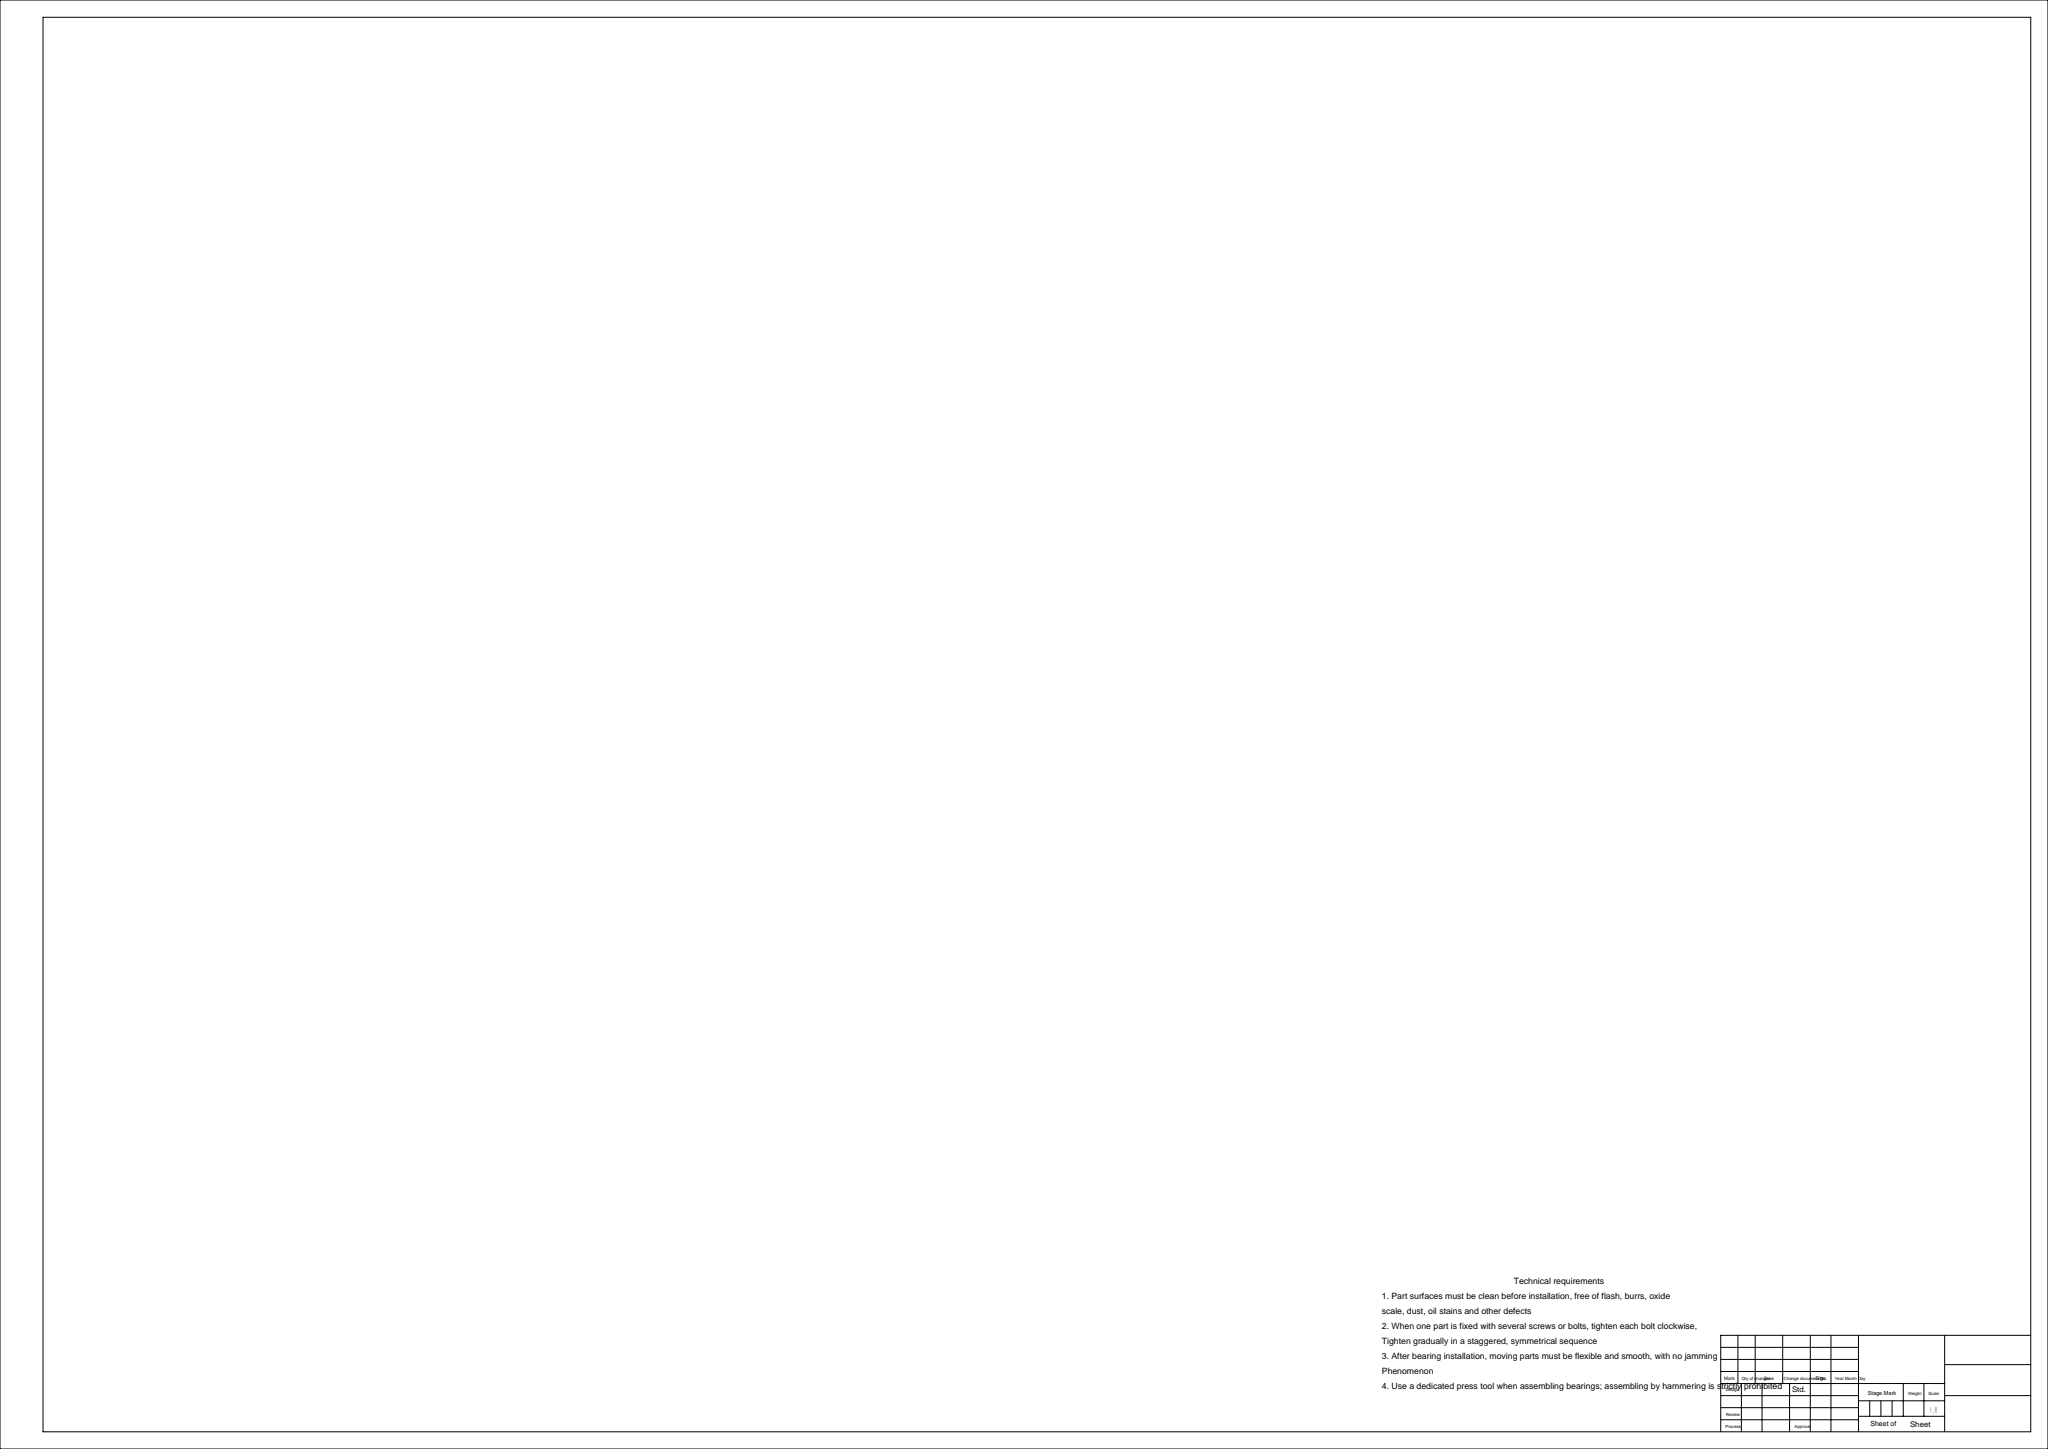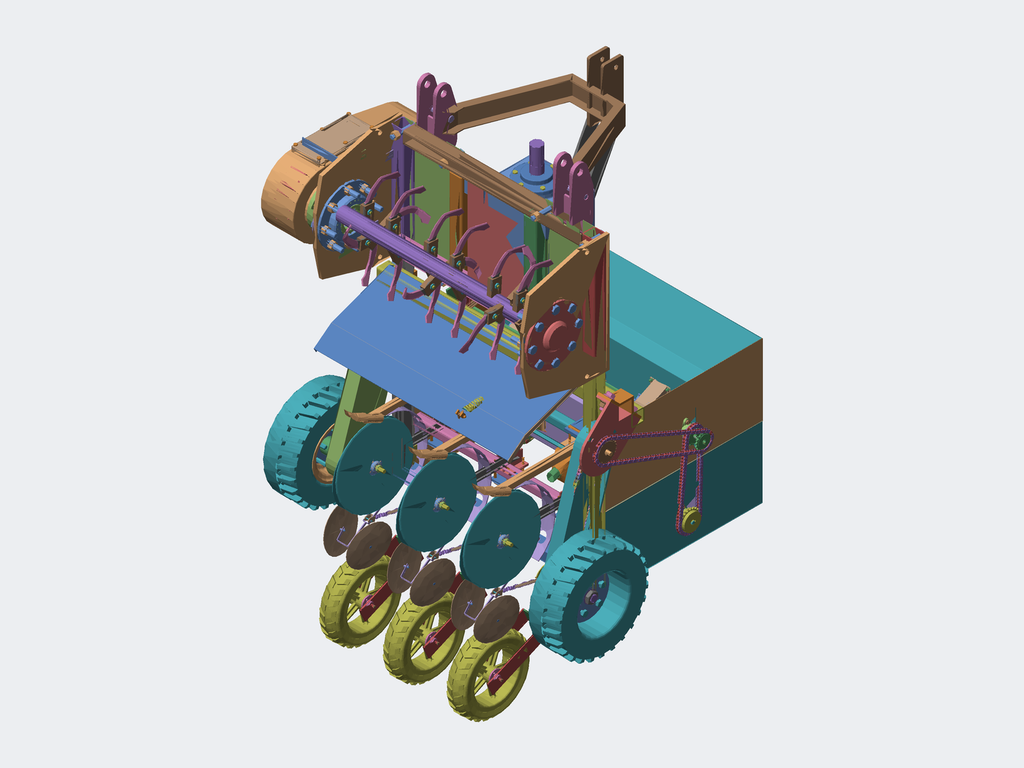Assembly | SolidWorks | 209 different items | 1308 placed
Parts list (item | name | quantity | parent item | size | volume | features):
1 | (subassembly) | x1 | - | - | - | features CompositeCurve 6
2 | (subassembly) | x1 | - | 866 x 574.882 x 353.001 mm | 3236381 mm3 | features ReferencePattern 8, LocalLPattern 1
3 | (subassembly) | x1 | - | 866 x 581.033 x 134.332 mm | 1380836 mm3 | -
4 | (subassembly) | x3 | in 5 | 163 x 229.711 x 140 mm | 1064629 mm3 | features CompositeCurve 9, ReferencePattern 6, LocalCirPattern 2, MirrorCompFeat 1
5 | (subassembly) | x1 | - | - | 6401215 mm3 | features ReferencePattern 29, LocalLPattern 4, CompositeCurve 2, MirrorCompFeat 2, LocalCirPattern 1
6 | (subassembly) | x1 | - | - | - | features CompositeCurve 20
7 | (subassembly) | x3 | in 8 | 130 x 170 x 165 mm | 426747 mm3 | -
8 | (subassembly) | x1 | - | 338 x 752 x 1133 mm | 4481337 mm3 | features ReferencePattern 18, LocalLPattern 3, CompositeCurve 2, LocalCirPattern 1
9 | (subassembly) | x1 | - | - | - | -
10 | (subassembly) | x1 | - | - | - | features ReferencePattern 8, LocalCirPattern 2, CompositeCurve 1
11 | (subassembly) | x1 | - | - | 19308799 mm3 | features ReferencePattern 66, LocalCirPattern 6, LocalLPattern 2, CompositeCurve 1, MirrorCompFeat 1
12 | (subassembly) | x3 | in 18 | 109 x 450 x 60 mm | 238814 mm3 | features CompositeCurve 2, MirrorCompFeat 2, ReferencePattern 2
13 | (subassembly) | x3 | - | 168.807 x 189.61 x 405.761 mm | 223720 mm3 | features CompositeCurve 6, MirrorCompFeat 2, ReferencePattern 2
14 | (subassembly) | x1 | in 5 | 105 x 105 x 103.075 mm | 214366 mm3 | features CompositeCurve 2
15 | (subassembly) | x1 | - | - | 206432 mm3 | features ReferencePattern 96, Belt 1, LocalChainPattern 1
16 | (subassembly) | x1 | - | - | 364523 mm3 | features ReferencePattern 73, Belt 1, LocalChainPattern 1
17 | (subassembly) | x74 | in 16 | 36.351 x 17.823 x 16.175 mm | 2555 mm3 | -
18 | (subassembly) | x3 | - | 130 x 571.206 x 341.736 mm | 2047297 mm3 | features CompositeCurve 1, MirrorCompFeat 1, ReferencePattern 1
19 | (subassembly) | x1 | - | 510.982 x 565.982 x 357 mm | 19755634 mm3 | features ReferencePattern 5, CompositeCurve 3, LocalCirPattern 1
20 | (subassembly) | x35 | in 21 | - | - | -
21 | (subassembly) | x1 | - | 975 x 434.394 x 418.8 mm | 2976475 mm3 | features ReferencePattern 52, CompositeCurve 10, LocalLPattern 4, LocalCirPattern 2, AEMSimFeature 1
22 | (subassembly) | x3 | in 2 | 353.001 x 130.927 x 574.882 mm | 819203 mm3 | features ReferencePattern 7, CompositeCurve 3, MirrorCompFeat 2
23 | (subassembly) | x1 | in 10 | - | - | features CompositeCurve 47, AEMSimFeature 1
24 | (subassembly) | x49 | in 15 | 25.03 x 12.33 x 14.51 mm | 799.359 mm3 | -
25 | (subassembly) | x1 | in 10 | - | - | features CompositeCurve 84, AEMSimFeature 1, Belt 1
26 | - | x2 | in 19 | 95.5 x 93.873 x 2.5 mm | 3834 mm3 | features Extrusion 1
27 | - | x2 | in 23, 25 | - | - | features ICE 2, Extrusion 1, SweepThread 1
28 | - | x1 | in 25 | 660 x 205 x 60 mm | 1732722 mm3 | features ICE 2, Extrusion 1
29 | - | x2 | in 23, 25 | 250 x 200 x 60 mm | 547961 mm3 | features ICE 3, Cut 1, Extrusion 1
30 | - | x1 | in 23 | - | 127327 mm3 | features Boss 3, CurvePattern 2, Chamfer 1, CompositeCurve 1, Extrusion 1, MirrorPattern 1, MirrorSolid 1
31 | - | x2 | in 23, 25 | 32 x 32 x 76 mm | 32270 mm3 | features Helix 1, Sweep 1
32 | - | x3 | in 4 | 115 x 115 x 40 mm | 37157 mm3 | features ICE 5, Extrusion 1, RefAxis 1, RefPoint 1
33 | - | x3 | in 4 | 120 x 120 x 7.5 mm | 38485 mm3 | features RefAxis 4, ICE 2, Extrusion 1
34 | - | x3 | in 4 | 98.826 x 98.952 x 30 mm | 216398 mm3 | features Extrusion 1, ICE 1
35 | - | x3 | in 4 | 100 x 100 x 65 mm | 446877 mm3 | features ICE 2, CirPattern 1, Extrusion 1
36 | - | x2 | - | 260 x 260 x 30 mm | 552397 mm3 | features ICE 2, Chamfer 1, Extrusion 1
37 | - | x2 | in 19 | 49 x 53.209 x 1.5 mm | 876.142 mm3 | features Extrusion 1
38 | - | x1 | - | 260 x 260 x 10 mm | 427257 mm3 | features Extrusion 1, ICE 1
39 | - | x246 | in 17, 24 | 25.03 x 12.33 x 1.665 mm | 399.679 mm3 | features Cut 1, Extrusion 1
40 | - | x1 | in 10 | 26 x 26 x 10 mm | 3542 mm3 | features Extrusion 1
41 | - | x1 | in 21 | 975 x 80 x 80 mm | 1427415 mm3 | features Chamfer 3, ICE 3, Extrusion 1, Fillet 1
42 | - | x11 | in 21 | 167.64 x 57.038 x 10 mm | 39018 mm3 | features Blend 1, Extrusion 1
43 | - | x18 | in 21 | 186.248 x 81.99 x 35.546 mm | 40697 mm3 | features ICE 2, Chamfer 1, CombineBodies 1, Deform 1, DeleteBody 1, Extrusion 1, FillRefSurface 1, MirrorPattern 1, RefCurve 1, Split 1, SurfCut 1, SweepCut 1
44 | - | x1 | in 25 | 64 x 64 x 195 mm | 414709 mm3 | features ICE 5, SweepThread 2, Chamfer 1, Extrusion 1
45 | - | x3 | in 3 | 134.332 x 42 x 580 mm | 122750 mm3 | features ICE 5, Blend 1, Extrusion 1
46 | - | x12 | in 2, 3 | 100 x 70 x 10 mm | 18547 mm3 | features Helix 2, SweepCut 2, Fillet 1, Sweep 1
47 | - | x9 | in 2, 3 | 100 x 80 x 10 mm | 76199 mm3 | features Extrusion 1
48 | - | x2 | in 19 | 34 x 14 x 9 mm | 3893 mm3 | features Extrusion 1, Fillet 1
49 | - | x1 | in 2 | 866 x 40 x 40 mm | 463134 mm3 | features WeldMemberFeat 1, WeldmentFeature 1
50 | - | x1 | in 3 | 866 x 40 x 40 mm | 463134 mm3 | features WeldMemberFeat 1, WeldmentFeature 1
51 | - | x3 | - | 12 x 280 x 12 mm | 31370 mm3 | features Extrusion 1, ICE 1, MirrorPattern 1
52 | - | x1 | - | 52.165 x 415.629 x 914 mm | 1472368 mm3 | features FlatPattern 2, SMBaseFlange 2, SheetMetal 2, ICE 1, MirrorSolid 1
53 | - | x5 | - | 130 x 60 x 57 mm | 96959 mm3 | features Cut 1, Extrusion 1, Fillet 1, ICE 1, LPattern 1
54 | - | x2 | - | 20 x 20 x 20 mm | 2749 mm3 | features Extrusion 1
55 | - | x4 | - | 16 x 26 x 5 mm | 1550 mm3 | features Extrusion 1
56 | - | x2 | - | 32 x 32 x 306 mm | 76200 mm3 | features Helix 1, RefAxis 1, Sweep 1
57 | - | x3 | in 22 | 328.42 x 176 x 80 mm | 44356 mm3 | features ICE 4, ExtruRefSurface 1, Thicken 1
58 | - | x1 | in 14 | 105 x 105 x 30 mm | 95976 mm3 | features ICE 2, Extrusion 1
59 | - | x1 | - | 10 x 5 x 5 mm | 221.448 mm3 | features Extrusion 1, Fillet 1
60 | - | x3 | in 7 | 22 x 22 x 165 mm | 19772 mm3 | features Extrusion 1, ICE 1
61 | - | x3 | in 7 | 68 x 68 x 120 mm | 167321 mm3 | features ICE 2, Extrusion 1
62 | - | x3 | in 7 | 130 x 170 x 96 mm | 239654 mm3 | features ICE 8, Blend 1, Extrusion 1, Shell 1
63 | - | x1 | in 8 | 15 x 15 x 1130 mm | 199245 mm3 | features ICE 3, Extrusion 1
64 | - | x3 | in 4 | 163 x 141.711 x 140 mm | 274719 mm3 | features ICE 8, Fillet 6, Extrusion 1, Shell 1
65 | - | x1 | in 5 | 45 x 45 x 15 mm | 8861 mm3 | features ICE 2, Extrusion 1
66 | - | x1 | in 14 | 48 x 48 x 7 mm | 4020 mm3 | features Extrusion 1, ICE 1
67 | - | x1 | in 14 | 55 x 55 x 10 mm | 12395 mm3 | features Extrusion 1
68 | - | x1 | in 14 | 75 x 75 x 103 mm | 101976 mm3 | features ICE 4, Extrusion 1, Shell 1
69 | - | x1 | in 5 | 15 x 15 x 1090 mm | 192288 mm3 | features ICE 2, Extrusion 1, Fillet 1
70 | - | x2 | in 5, 8 | 14 x 5 x 5 mm | 320.899 mm3 | features Extrusion 1, Fillet 1
71 | - | x1 | in 8 | 105 x 105 x 30 mm | 95568 mm3 | features ICE 2, Extrusion 1
72 | - | x1 | in 8 | 48 x 48 x 7 mm | 4020 mm3 | features Extrusion 1, ICE 1
73 | - | x1 | in 8 | 55 x 55 x 10 mm | 12395 mm3 | features Extrusion 1
74 | - | x1 | in 8 | 75 x 75 x 103 mm | 101976 mm3 | features ICE 4, Extrusion 1, Shell 1
75 | - | x2 | - | 580 x 21 x 21 mm | 191345 mm3 | features ICE 4, Revolution 1
76 | - | x3 | in 22 | 100 x 60 x 80 mm | 110678 mm3 | features ICE 3, Extrusion 1, MirrorPattern 1
77 | - | x3 | in 4 | 42.184 x 46.319 x 39 mm | 4653 mm3 | features Extrusion 1, ICE 1, Shell 1, Sweep 1
78 | - | x2 | - | 260 x 260 x 41 mm | 859714 mm3 | features ICE 3, Chamfer 2, CirPattern 1, Extrusion 1, Fillet 1
79 | - | x1 | - | 960 x 60 x 1436 mm | 5295924 mm3 | features ICE 2, MirrorPattern 2, LPattern 1, WeldMemberFeat 1, WeldmentFeature 1
80 | - | x6 | in 12 | 5 x 300 x 60 mm | 89607 mm3 | features Extrusion 1, ICE 1
81 | - | x2 | in 11 | 16 x 80 x 80 mm | 32317 mm3 | features Revolution 6, CirPattern 2, RevCut 2, MirrorPattern 1
82 | - | x3 | in 12 | 99 x 5 x 60 mm | 29700 mm3 | features Extrusion 1
83 | - | x6 | in 12 | 2 x 150 x 50 mm | 14950 mm3 | features ICE 3, Extrusion 1
84 | - | x12 | in 5 | 50 x 9.031 x 30 mm | 3952 mm3 | features ICE 2, Extrusion 1
85 | - | x3 | in 4 | 80 x 45 x 5 mm | 16384 mm3 | features ICE 3, Extrusion 1, LPattern 1
86 | - | x2 | - | 80 x 40 x 40 mm | 37542 mm3 | features Extrusion 1, ICE 1, MirrorSolid 1
87 | - | x3 | - | 34 x 10 x 14 mm | 1005 mm3 | features Extrusion 1, ICE 1, MirrorSolid 1
88 | - | x2 | - | 530 x 2 x 280 mm | 290567 mm3 | features ICE 2, Extrusion 1
89 | - | x1 | - | 415.5 x 2 x 290 mm | 240990 mm3 | features Extrusion 1
90 | - | x1 | in 5 | 337 x 313.5 x 920 mm | 1609120 mm3 | features MirrorPattern 2, FlatPattern 1, ICE 1, SMBaseFlange 1, SheetMetal 1
91 | - | x1 | in 5 | 32 x 752 x 333 mm | 518361 mm3 | features FlatPattern 1, ICE 1, SMBaseFlange 1, SheetMetal 1
92 | - | x1 | in 10 | 5 x 24 x 24 mm | 880.809 mm3 | features Revolution 5, CirPattern 2, RevCut 2
93 | - | x1 | in 5 | 32 x 752 x 333 mm | 518481 mm3 | features ICE 2, FlatPattern 1, SMBaseFlange 1, SheetMetal 1
94 | - | x3 | in 22 | 35 x 12 x 415 mm | 167863 mm3 | features Extrusion 1, ICE 1
95 | - | x1 | - | 40 x 10 x 69.01 mm | 22746 mm3 | features Extrusion 1
96 | - | x1 | - | 40 x 10 x 66.57 mm | 21770 mm3 | features Extrusion 1
97 | - | x1 | in 8 | 32 x 752 x 337 mm | 524643 mm3 | features FlatPattern 1, ICE 1, SMBaseFlange 1, SheetMetal 1
98 | - | x1 | in 8 | 32 x 752 x 337 mm | 524731 mm3 | features ICE 2, FlatPattern 1, SMBaseFlange 1, SheetMetal 1
99 | - | x1 | - | 60 x 60 x 200 mm | 299813 mm3 | features ICE 2, Extrusion 1
100 | - | x1 | in 8 | 337 x 313.5 x 920 mm | 1639360 mm3 | features MirrorPattern 2, FlatPattern 1, ICE 1, SMBaseFlange 1, SheetMetal 1
101 | - | x3 | - | 16 x 16 x 176 mm | 26240 mm3 | features Helix 1, RefAxis 1, Sweep 1
102 | - | x3 | - | 20 x 232 x 20 mm | 18563 mm3 | features ICE 5, Extrusion 1
103 | - | x6 | in 18 | 9 x 30 x 30 mm | 4054 mm3 | features Revolution 5, CirPattern 2, RevCut 2
104 | - | x3 | in 13 | 138.916 x 10 x 352 mm | 16665 mm3 | features ICE 6, Extrusion 1, MirrorPattern 1
105 | - | x6 | in 13 | 189.61 x 7.325 x 189.61 mm | 102683 mm3 | features Fillet 1, ICE 1, Revolution 1
106 | - | x3 | in 18 | 87.248 x 341.454 x 341.945 mm | 1756971 mm3 | features CirPattern 5, ICE 5, Fillet 3, Chamfer 2, Revolution 2
107 | - | x6 | in 18 | 60 x 60 x 18.5 mm | 16720 mm3 | features ICE 2, Extrusion 1
108 | - | x2 | in 23, 25 | 240 x 240 x 140 mm | 3010326 mm3 | features ICE 4, Extrusion 1, Fillet 1, MirrorPattern 1
109 | - | x2 | in 23, 25 | 440 x 440 x 140 mm | 12462431 mm3 | features BlendCut 2, CirPattern 2, Extrusion 1, Fillet 1
110 | - | x1 | in 23 | 48 x 48 x 10 mm | 5529 mm3 | features Extrusion 1
111 | - | x1 | in 25 | 48 x 48 x 10 mm | 5529 mm3 | features Extrusion 1
112 | - | x3 | in 18 | 10 x 10 x 130 mm | 9964 mm3 | features Extrusion 1, ICE 1
113 | - | x2 | - | 300 x 98 x 92 mm | 689780 mm3 | features ICE 2, Extrusion 1, Fillet 1, LPattern 1
114 | - | x4 | in 19 | 20 x 90 x 90 mm | 55631 mm3 | features Revolution 6, CirPattern 2, RevCut 2, MirrorPattern 1
115 | - | x1 | - | 550 x 539.301 x 285 mm | 1145728 mm3 | features ICE 3, MirrorSolid 3, ExtruRefSurface 1, Thicken 1
116 | - | x2 | - | 341.614 x 178.454 x 10 mm | 201659 mm3 | features Extrusion 1
117 | - | x3 | - | 30 x 95 x 165 mm | 47978 mm3 | features ICE 1, WeldMemberFeat 1, WeldmentFeature 1
118 | - | x7 | - | 53.74 x 83.25 x 20 mm | 11198 mm3 | features ICE 2, Extrusion 1
119 | - | x3 | - | 17 x 17 x 154 mm | 7958 mm3 | features Helix 1, RefAxis 1, Sweep 1
120 | - | x2 | in 11 | 20 x 90 x 90 mm | 55631 mm3 | features Revolution 6, CirPattern 2, RevCut 2, MirrorPattern 1
121 | - | x3 | - | 4 x 4 x 50 mm | 613.938 mm3 | features Chamfer 1, Cut 1, Extrusion 1
122 | - | x1 | in 11 | 21 x 100 x 100 mm | 73176 mm3 | features Revolution 6, CirPattern 2, RevCut 2, MirrorPattern 1
123 | - | x3 | in 11 | 25 x 100 x 100 mm | 96597 mm3 | features Revolution 6, CirPattern 2, RevCut 2, MirrorPattern 1
124 | - | x1 | in 5 | 13.2 x 35 x 35 mm | 6194 mm3 | features Revolution 4, CirPattern 1
125 | - | x2 | - | 26 x 140 x 140 mm | 191182 mm3 | features Revolution 3, CirPattern 1
126 | - | x6 | in 22 | 22 x 40 x 40 mm | 10628 mm3 | features Revolution 3, RevCut 2, CirPattern 1
127 | - | x1 | in 10 | 26.17 x 22.664 x 15.9 mm | 3864 mm3 | features Cut 2, Chamfer 1, Extrusion 1
128 | - | x26 | - | 32.95 x 28.536 x 19 mm | 7406 mm3 | features Cut 2, Chamfer 1, Extrusion 1
129 | - | x4 | in 19 | 36.4 x 18.475 x 16 mm | 3739 mm3 | features RevCut 4, Chamfer 1, Extrusion 1, Fillet 1, LPattern 1, Revolution 1
130 | - | x14 | in 19 | 41.4 x 18.475 x 16 mm | 4131 mm3 | features RevCut 4, Chamfer 1, Extrusion 1, Fillet 1, LPattern 1, Revolution 1
131 | - | x31 | in 11 | 37.5 x 20.785 x 18 mm | 5444 mm3 | features RevCut 4, Chamfer 1, Extrusion 1, Fillet 1, LPattern 1, Revolution 1
132 | - | x2 | - | 34.5 x 14 x 14 mm | 2728 mm3 | features Chamfer 1, Cut 1, Fillet 1, Revolution 1
133 | - | x40 | in 5, 8 | 25.3 x 15.011 x 13 mm | 1760 mm3 | features RevCut 4, Chamfer 1, Extrusion 1, Fillet 1, LPattern 1, Revolution 1
134 | - | x6 | in 11 | 35.3 x 15.011 x 13 mm | 2262 mm3 | features RevCut 4, Chamfer 1, Extrusion 1, Fillet 1, LPattern 1, Revolution 1
135 | - | x10 | in 10 | 75 x 27.713 x 24 mm | 17949 mm3 | features RevCut 4, Chamfer 1, Extrusion 1, Fillet 1, LPattern 1, Revolution 1
136 | - | x24 | - | 102.5 x 34.641 x 30 mm | 37820 mm3 | features RevCut 4, Chamfer 1, Extrusion 1, Fillet 1, LPattern 1, Revolution 1
137 | - | x18 | in 21 | 37.5 x 20.785 x 18 mm | 5444 mm3 | features RevCut 4, Chamfer 1, Extrusion 1, Fillet 1, LPattern 1, Revolution 1
138 | - | x18 | in 21 | 17.386 x 20.03 x 10.8 mm | 1566 mm3 | features Cut 2, Chamfer 1, Extrusion 1
139 | - | x12 | in 5 | 12.482 x 14.38 x 4 mm | 327.094 mm3 | features Cut 2, Chamfer 1, Extrusion 1
140 | - | x6 | in 22 | 23.219 x 26.75 x 8 mm | 2049 mm3 | features Cut 2, Chamfer 1, Extrusion 1
141 | - | x4 | in 5, 8 | 26 x 16 x 16 mm | 2579 mm3 | features Cut 1, LPattern 1, RevCut 1, Revolution 1
142 | - | x8 | in 5, 8 | 23.9 x 10 x 10 mm | 819.417 mm3 | features Cut 1, LPattern 1, RevCut 1, Revolution 1
143 | - | x2 | - | 124 x 28 x 28 mm | 46998 mm3 | features Chamfer 1, Cut 1, Fillet 1, Revolution 1
144 | - | x24 | in 4 | 16 x 15.8 x 15.673 mm | 989.006 mm3 | features Chamfer 1, Cut 1, LPattern 1, RevCut 1, Revolution 1
145 | - | x2 | in 5, 8 | 99 x 61 x 32.9 mm | 62248 mm3 | features Revolution 5, Boss 2, RevCut 2, CirPattern 1, Cut 1, Extrusion 1
146 | - | x6 | in 4 | 30.97 x 16 x 16 mm | 2140 mm3 | features BlendCut 1, LPattern 1, MirrorPattern 1, RevCut 1, Revolution 1
147 | - | x31 | in 11 | 18.367 x 18.334 x 3.1 mm | 444.091 mm3 | features Extrusion 1
148 | - | x6 | in 11 | 12.277 x 12.254 x 2.1 mm | 135.755 mm3 | features Extrusion 1
149 | - | x24 | in 22 | 14.968 x 7.7 x 7.7 mm | 225.537 mm3 | features Cut 1, Fillet 1, Revolution 1
150 | - | x1 | in 11 | 11 x 18 x 12.702 mm | 898.381 mm3 | features Boss 1, Revolution 1
151 | - | x1 | in 11 | 688 x 310 x 170 mm | 8954968 mm3 | features 3DProfileFeature 6, HoleWzd 6, ICE 6, CirPattern 4, Fillet 3, MirrorPattern 3, Cut 1, Extrusion 1
152 | - | x1 | in 11 | 134.581 x 133.659 x 70 mm | 542357 mm3 | features ICE 2, CirPattern 1, Extrusion 1, RefAxis 1
153 | - | x1 | in 11 | 260.857 x 260.456 x 75 mm | 1917959 mm3 | features ICE 6, Chamfer 5, CirPattern 2, MirrorPattern 2, Extrusion 1, RefAxis 1, RevCut 1
154 | - | x2 | - | 99 x 28 x 28 mm | 37494 mm3 | features Chamfer 1, Cut 1, Fillet 1, Revolution 1
155 | - | x1 | in 11 | 268.959 x 268.959 x 75 mm | 2318333 mm3 | features Chamfer 5, ICE 5, CirPattern 2, Extrusion 1, MirrorPattern 1, RefAxis 1, RevCut 1
156 | - | x1 | in 11 | 62 x 62 x 310 mm | 627287 mm3 | features ICE 4, Chamfer 2, CirPattern 1, Extrusion 1, SweepCut 1
157 | - | x1 | in 11 | 50 x 50 x 160 mm | 295367 mm3 | features ICE 2, Chamfer 1, Extrusion 1
158 | - | x1 | in 11 | 68 x 68 x 312.5 mm | 737851 mm3 | features ICE 4, Chamfer 1, CirPattern 1, Extrusion 1, SweepCut 1
159 | - | x1 | in 11 | 23 x 170 x 170 mm | 323268 mm3 | features Chamfer 1, CirPattern 1, ICE 1, Revolution 1
160 | - | x1 | in 11 | 23 x 190 x 190 mm | 393528 mm3 | features Chamfer 1, CirPattern 1, ICE 1, Revolution 1
161 | - | x1 | in 11 | 40 x 170 x 170 mm | 559070 mm3 | features CirPattern 3, ICE 3, 3DProfileFeature 1, HoleWzd 1, Revolution 1
162 | - | x3 | in 11 | 18 x 170 x 170 mm | 307921 mm3 | features Chamfer 1, CirPattern 1, ICE 1, Revolution 1
163 | - | x2 | in 11 | 63 x 63 x 20 mm | 22197 mm3 | features Chamfer 1, Extrusion 1
164 | - | x2 | in 11 | 63 x 63 x 23.5 mm | 27024 mm3 | features Chamfer 1, Extrusion 1
165 | - | x6 | - | 17.5 x 6 x 6 mm | 227.981 mm3 | features Chamfer 1, Cut 1, Fillet 1, Revolution 1
166 | - | x1 | in 11 | 39 x 190 x 190 mm | 716899 mm3 | features CirPattern 3, ICE 3, 3DProfileFeature 1, HoleWzd 1, Revolution 1
167 | - | x2 | in 11 | 70 x 70 x 17.5 mm | 39425 mm3 | features Chamfer 1, Extrusion 1
168 | - | x1 | in 11 | 270 x 130 x 13 mm | 385260 mm3 | features Extrusion 1, Fillet 1, ICE 1
169 | - | x1 | in 19 | 380 x 380 x 282 mm | 14746846 mm3 | features ICE 13, 3DProfileFeature 3, HoleWzd 3, Fillet 2, Extrusion 1
170 | - | x1 | in 19 | 180 x 180 x 85 mm | 1041607 mm3 | features ICE 4, Fillet 2, 3DProfileFeature 1, CirPattern 1, Extrusion 1, HoleWzd 1
171 | - | x1 | in 19 | 155.563 x 155.563 x 25 mm | 236034 mm3 | features ICE 2, Extrusion 1, Fillet 1
172 | - | x1 | in 19 | 260 x 260 x 75 mm | 829791 mm3 | features ICE 2, Extrusion 1, Fillet 1
173 | - | x1 | in 19 | 329.5 x 60 x 60 mm | 697643 mm3 | features ICE 3, Chamfer 2, Revolution 1
174 | - | x1 | in 19 | 274.5 x 60 x 60 mm | 542135 mm3 | features ICE 3, Chamfer 2, Revolution 1
175 | - | x2 | in 19 | 45.295 x 166.152 x 166.786 mm | 471542 mm3 | features BlendCut 1, CirPattern 1, ICE 1, RefAxis 1, Revolution 1
176 | - | x6 | - | 31.5 x 6 x 6 mm | 403.91 mm3 | features Chamfer 1, Cut 1, Fillet 1, Revolution 1
177 | - | x1 | in 19 | 180 x 180 x 35 mm | 406222 mm3 | features ICE 2, Extrusion 1, Fillet 1
178 | - | x1 | in 25 | 12 x 12 x 19.5 mm | 659.077 mm3 | features Chamfer 2, Cut 2, Boss 1, Extrusion 1, Fillet 1, LPattern 1, RevCut 1
179 | - | x4 | in 23, 25 | 57.7 x 43 x 43 mm | 28324 mm3 | features Fillet 2, RevCut 2, Boss 1, Chamfer 1, Extrusion 1, LPattern 1, Revolution 1
180 | - | x2 | in 23 | 53.116 x 46 x 15 mm | 17946 mm3 | features RevCut 2, Chamfer 1, Extrusion 1, LPattern 1
181 | - | x2 | in 25 | 53.116 x 46 x 15 mm | 18987 mm3 | features RevCut 2, Chamfer 1, Extrusion 1, LPattern 1
182 | - | x1 | in 23 | 26.58 x 18.163 x 15.73 mm | 2955 mm3 | features RevCut 3, Boss 1, Chamfer 1, Extrusion 1, Fillet 1, LPattern 1
183 | - | x4 | in 23, 25 | 42.8 x 42.8 x 20 mm | 13089 mm3 | features RevCut 3, Extrusion 1, Fillet 1, LPattern 1, Revolution 1
184 | - | x3 | in 4 | 121.759 x 70.429 x 82 mm | 20309 mm3 | features MirrorPattern 8, ICE 6, Blend 1, Fillet 1, RefAxis 1, Shell 1
185 | - | x2 | in 23 | 28 x 28 x 10 mm | 3016 mm3 | features Extrusion 1
186 | - | x2 | in 25 | 28 x 28 x 10 mm | 3016 mm3 | features Extrusion 1
187 | - | x6 | in 13 | 28 x 10 x 10 mm | 844.638 mm3 | features Chamfer 1, Cut 1, Fillet 1, Revolution 1
188 | - | x1 | - | 9.37 x 98.633 x 98.858 mm | 54827 mm3 | features Chamfer 3, Cut 2, Revolution 2, CirPattern 1
189 | - | x1 | in 15 | 9.37 x 98.633 x 98.858 mm | 53510 mm3 | features Chamfer 3, Cut 2, Revolution 2, CirPattern 1
190 | - | x2 | in 15, 16 | 9.37 x 73.539 x 73.841 mm | 27730 mm3 | features Chamfer 3, Cut 2, Revolution 2, CirPattern 1
191 | - | x2 | - | 555.5 x 409.096 x 15 mm | 2756721 mm3 | features ICE 5, Chamfer 1, CirPattern 1, Extrusion 1, MirrorPattern 1
192 | - | x123 | in 15, 17 | 24.77 x 12.07 x 16.175 mm | 1756 mm3 | features Boss 2, Chamfer 1, Extrusion 1, MirrorPattern 1
193 | - | x18 | in 21 | 70.526 x 45 x 21 mm | 38872 mm3 | features ICE 3, Extrusion 1
194 | - | x17 | in 21 | 167.64 x 57.038 x 10 mm | 39018 mm3 | features MirrorStock 1
195 | - | x1 | in 23 | 64 x 64 x 195 mm | 414708 mm3 | features ICE 5, SweepThread 2, Chamfer 1, Extrusion 1
196 | - | x2 | - | 200 x 100 x 30 mm | 64241 mm3 | features WeldMemberFeat 1, WeldmentFeature 1
197 | - | x3 | - | 100 x 100 x 30 mm | 41483 mm3 | features WeldMemberFeat 1, WeldmentFeature 1
198 | - | x4 | in 11 | 85.5 x 83.408 x 2.5 mm | 3180 mm3 | features Extrusion 1
199 | - | x2 | - | 30 x 2 x 30 mm | 720.996 mm3 | features Extrusion 1
200 | - | x6 | in 22 | 350 x 350 x 2.3 mm | 217251 mm3 | features ICE 3, Extrusion 1, Sweep 1
201 | - | x3 | in 22 | 130.429 x 28.183 x 19 mm | 26177 mm3 | features ICE 2, Sweep 1
202 | - | x6 | in 22 | 62 x 14 x 62 mm | 4234 mm3 | features ICE 2, Revolution 1
203 | - | x1 | in 10 | 20 x 20 x 120 mm | 27495 mm3 | features ICE 5, Extrusion 1
204 | - | x3 | in 16, 23, 25 | 30 x 98.633 x 98.858 mm | 147727 mm3 | features ICE 2, CirPattern 1, Cut 1, RefAxis 1, Revolution 1
205 | - | x2 | in 23, 25 | 30 x 98.633 x 98.858 mm | 118578 mm3 | features ICE 2, CirPattern 1, Cut 1, RefAxis 1, Revolution 1
206 | - | x1 | in 23 | 660 x 205 x 50 mm | 1585598 mm3 | features ICE 2, Extrusion 1
207 | - | x2 | in 23, 25 | 148.492 x 148.492 x 60 mm | 135835 mm3 | features Cut 1, Extrusion 1, ICE 1
208 | - | x2 | in 23, 25 | 200 x 200 x 20 mm | 321867 mm3 | features Extrusion 1, ICE 1
209 | - | x1 | in 10 | 1200 x 60 x 60 mm | 1025756 mm3 | features WeldMemberFeat 1, WeldmentFeature 1
Mates (type | each side: item.copy, entity, surface, feature), first 427 of 1009 lines:
In the top assembly
Coincident | 79.1 plane | assembly plane | 2 times
Coincident | assembly axis | assembly axis | 15 times
Coincident | assembly face | assembly face | 9 times
Coincident | 79.1 face plane Gb/6728-1986方形空心型钢 060 X 60 X 4(1) | 91.1 face plane Base-Flange 1 | 3 times
Coincident | 79.1 face plane Gb/6728-1986方形空心型钢 060 X 60 X 4(1) | 49.1 face plane Gb/6728-1986方形空心型钢 040 X 40 X 4(1)
Coincident | 79.1 edge | 91.1 edge
Tangent | assembly face | assembly face
Coincident | assembly plane | assembly plane | 3 times
Coincident | 79.1 face plane Gb/6728-1986方形空心型钢 060 X 60 X 4(1) | assembly face | 7 times
Coincident | assembly axis | 199.1 axis
Coincident | assembly face | 199.1 face plane Boss-Extrude 1
Coincident | assembly plane | 79.1 plane
Coincident | 2.1 plane | assembly plane
Coincident | 79.1 face plane Gb/6728-1986方形空心型钢 060 X 60 X 4(1) | 50.1 face plane Gb/6728-1986方形空心型钢 040 X 40 X 4(1)
Coincident | 3.1 plane | assembly plane
Coincident | 79.1 plane | 19.1 plane
Coincident | 79.1 face plane Gb/6728-1986方形空心型钢 060 X 60 X 4(1) | 169.1 face plane Boss-Extrude 1
Coincident | 19.1 plane | assembly plane | 2 times
Coincident | 79.1 edge | 19.1 plane
Coincident | 173.1 axis | 99.1 axis
Coincident | 173.1 edge | 99.1 edge
Coincident | 173.1 face plane Revolve 1 | 99.1 face plane Cut-Extrude 1
Coincident | 99.1 axis | 156.1 axis
Coincident | 99.1 face plane Cut-Extrude 2 | 156.1 face plane Boss-Extrude 4
Coincident | 158.1 axis | 41.1 axis
Coincident | 158.1 face plane Boss-Extrude 3 | 41.1 face plane Boss-Extrude 1
Coincident | 41.1 axis | 191.1 axis
Coincident | 79.1 face plane Gb/6728-1986方形空心型钢 060 X 60 X 4(1) | 191.1 edge
Parallel | assembly plane | 191.1 plane
Coincident | 158.1 axis | 78.1 axis
Coincident | 125.1 axis | 158.1 axis
Coincident | 78.1 face plane Boss-Extrude 1 | 125.1 face plane Base-Revolve
Coincident | 125.2 axis | 36.1 axis
Coincident | 191.1 axis | 36.1 axis
Coincident | 78.2 axis | 36.1 axis
Coincident | 191.1 face plane Boss-Extrude 1 | 36.1 face plane Boss-Extrude 1
Coincident | 158.1 axis | 38.1 axis
Coincident | 78.1 axis | 38.1 axis
Coincident | 19.1 plane | 11.1 plane
Coincident | 191.2 axis | 191.1 axis | 2 times
Coincident | 79.1 face plane Gb/6728-1986方形空心型钢 060 X 60 X 4(1) | 191.2 face plane Boss-Extrude 1
Coincident | 52.1 face plane Mirror 3 | 55.1 face plane Boss-Extrude 1
Parallel | 52.1 edge | 55.1 edge
Coincident | 52.1 face plane Mirror 3 | assembly face
Coincident | 52.1 face plane Mirror 3 | 55.2 face plane Boss-Extrude 1
Parallel | 52.1 edge | 55.2 edge
DistanceDim | 55.1 face plane Boss-Extrude 1 | 55.2 face plane Boss-Extrude 1
Coincident | 55.1 axis | 55.2 axis
Coincident | 79.1 face plane Gb/6728-1986方形空心型钢 060 X 60 X 4(1) | 53.1 face plane LPattern 2
Coincident | 79.1 plane | 53.1 plane
DistanceDim | 53.1 face plane Boss-Extrude 1 | 53.2 face plane LPattern 2
Coincident | 53.1 axis | 86.1 axis
DistanceDim | 55.2 edge | 52.1 edge
Coincident | 75.1 axis | 86.1 axis
DistanceDim | 55.2 face plane Boss-Extrude 1 | 55.3 face plane Boss-Extrude 1
Parallel | 75.2 axis | 86.2 axis
Coincident | 191.2 face plane Boss-Extrude 1 | 38.1 face plane Boss-Extrude 1
Coincident | 191.2 face plane Cut-Extrude 1 | 78.1 face plane Boss-Extrude 1
Coincident | 191.1 face plane Cut-Extrude 1 | 78.2 face plane Boss-Extrude 1
Coincident | assembly edge | assembly plane
Parallel | 10.1 plane | assembly plane | 2 times
Coincident | 79.1 face plane Gb/6728-1986方形空心型钢 060 X 60 X 4(1) | 209.1 face plane Gb/6728-1986方形空心型钢 60 X 60 X 4(1)
Coincident | 79.1 face plane Gb/6728-1986方形空心型钢 060 X 60 X 4(1) | 53.3 face plane LPattern 2
Coincident | 79.1 plane | 53.3 plane
Coincident | 47.1 plane | 53.3 plane
Coincident | 83.1 axis | 53.3 axis
Coincident | 106.1 plane | 53.4 plane
Coincident | 27.1 axis | 95.1 axis
Coincident | 79.1 face plane Gb/6728-1986方形空心型钢 060 X 60 X 4(1) | 95.1 face plane Boss-Extrude 1
Coincident | 27.2 axis | 96.1 axis
Coincident | 95.1 face plane Boss-Extrude 1 | 96.1 face plane Boss-Extrude 1
Parallel | 79.1 face plane Gb/6728-1986方形空心型钢 060 X 60 X 4(1) | 96.1 face plane Boss-Extrude 1
Coincident | 83.2 axis | assembly axis | 2 times
Coincident | 53.3 axis | assembly axis
Coincident | 12.1 plane | assembly plane
Coincident | 51.1 axis | assembly axis
Coincident | 51.1 axis | 121.1 axis
Coincident | 83.3 axis | 121.1 axis
Coincident | 125.2 axis | 36.2 axis
Coincident | 191.1 axis | 36.2 axis
Coincident | 191.1 face plane Boss-Extrude 1 | 36.2 face plane Boss-Extrude 1
Parallel | 79.1 face plane Gb/6728-1986方形空心型钢 060 X 60 X 4(1) | 115.1 face plane 加厚1
Coincident | 19.1 plane | 115.1 plane
DistanceDim | assembly face | assembly face
Coincident | 79.1 face plane Gb/6728-1986方形空心型钢 060 X 60 X 4(1) | 113.1 face plane Boss-Extrude 1
Coincident | 79.1 face plane Gb/6728-1986方形空心型钢 060 X 60 X 4(1) | 113.1 face plane LPattern 1
Coincident | 115.1 axis | 113.1 axis
Coincident | 115.1 face plane 加厚1 | 113.1 face plane LPattern 1
Coincident | 115.1 axis | 116.1 axis
Coincident | 115.1 face plane Boss-Extrude 4 | 116.1 face plane Boss-Extrude 1
Coincident | 55.4 axis | 75.2 axis | 2 times
Coincident | 53.1 plane | 86.1 plane
Coincident | 55.1 axis | 75.1 axis
Coincident | 75.1 axis | 56.1 axis
Coincident | 75.1 face plane Boss-Extrude 3 | 199.1 face plane Boss-Extrude 1
Coincident | 56.1 axis | 199.1 axis
Coincident | 51.1 axis | 119.1 axis
Coincident | 27.2 axis | 128.1 axis
Coincident | 96.1 face plane Boss-Extrude 1 | 128.1 face plane Base-Extrude
Coincident | 27.1 axis | 128.2 axis
Coincident | 95.1 face plane Boss-Extrude 1 | 128.2 face plane Base-Extrude
Coincident | 36.2 face plane Boss-Extrude 1 | 136.1 face plane Base-Extrude
Coincident | 36.2 axis | 136.1 axis
Coincident | 136.1 axis | 128.3 axis
Coincident | 78.2 face plane Boss-Extrude 1 | 128.3 face plane Base-Extrude
Coincident | 78.1 axis | 136.2 axis
Coincident | 38.1 face plane Boss-Extrude 1 | 136.2 face plane Base-Extrude
Coincident | 136.3 axis | 128.4 axis
Coincident | 78.1 face plane Boss-Extrude 1 | 128.4 face plane Base-Extrude
Coincident | 79.1 axis | 88.1 axis | 2 times
Coincident | 79.1 face plane Gb/6728-1986方形空心型钢 060 X 60 X 4(1) | 88.1 face plane Boss-Extrude 1
Coincident | 88.1 face plane Boss-Extrude 1 | assembly face
Coincident | 88.1 axis | assembly axis
Coincident | 88.1 face plane Boss-Extrude 1 | 136.4 face plane Base-Extrude
Coincident | 88.1 axis | 136.4 axis
Coincident | 79.1 face plane Gb/6728-1986方形空心型钢 060 X 60 X 4(1) | 88.2 face plane Boss-Extrude 1
Coincident | 79.1 axis | 88.2 axis | 2 times
Coincident | 88.2 face plane Boss-Extrude 1 | 136.5 face plane Base-Extrude
Coincident | 79.1 axis | 136.5 axis
Coincident | 79.1 plane | 89.1 plane | 2 times
Coincident | 79.1 plane | 89.1 face plane Boss-Extrude 1
Coincident | 115.1 axis | assembly axis
Coincident | 115.1 face plane 加厚1 | assembly edge
Coincident | 115.1 axis | 154.1 axis
Coincident | 115.1 face plane 加厚1 | 154.1 edge
Coincident | 116.1 axis | 143.1 axis
Coincident | 116.1 face plane Boss-Extrude 1 | 143.1 edge
Coincident | 172.1 axis | 143.2 axis
Coincident | 116.1 face plane Boss-Extrude 1 | 143.2 edge
Parallel | 191.1 face plane Boss-Extrude 1 | 88.1 face plane Boss-Extrude 1
Coincident | 136.4 axis | 128.5 axis
Coincident | 79.1 face plane Gb/6728-1986方形空心型钢 060 X 60 X 4(1) | 128.5 face plane Base-Extrude
Tangent | 79.1 face plane Gb/6728-1986方形空心型钢 060 X 60 X 4(1) | 54.1 face cylinder Boss-Extrude 1
DistanceDim | 54.1 plane | 191.1 face plane Boss-Extrude 1
Coincident | 52.1 axis | 54.1 axis
DistanceDim | 54.1 plane | 79.1 face plane Gb/6728-1986方形空心型钢 060 X 60 X 4(1)
Coincident | 52.1 face plane Mirror 3 | 54.2 face plane Boss-Extrude 1
Coincident | 56.1 plane | 199.1 face plane Boss-Extrude 1
Coincident | 55.1 axis | 132.1 axis
Coincident | 55.2 face plane Boss-Extrude 1 | 132.1 edge
Coincident | 75.2 axis | 132.2 axis
Coincident | 145.1 axis | assembly axis
Coincident | 203.1 axis | assembly axis | 2 times
Coincident | 63.1 axis | 59.1 axis | 2 times
Coincident | 63.1 face plane Cut-Extrude 3 | 59.1 face plane Base-Extrude
Coincident | 79.1 face plane Gb/6728-1986方形空心型钢 060 X 60 X 4(1) | 98.1 face plane Base-Flange 1
Coincident | 90.1 face plane Base-Flange 1 | 100.1 face plane Base-Flange 1
Coincident | 100.1 plane | assembly plane
Coincident | 40.1 face plane Boss-Extrude 1 | assembly face
Coincident | 63.1 axis | 190.1 axis
Coincident | 63.1 axis | 190.2 axis
Coincident | 69.1 axis | 204.1 axis
Coincident | 145.1 face plane Boss-Extrude 2 | 204.1 face plane Boss-Extrude 1
Coincident | 203.1 axis | 189.1 axis
Coincident | 53.3 plane | 118.1 plane
Coincident | 79.1 face plane Gb/6728-1986方形空心型钢 060 X 60 X 4(1) | 118.1 face plane Boss-Extrude 1
Coincident | 118.1 axis | 176.1 axis
Coincident | 118.1 face plane Boss-Extrude 1 | 176.1 edge
Coincident | 191.2 face plane Boss-Extrude 1 | 196.1 face plane Gbt706-2008 热轧等边角钢 030×4(1)
Parallel | 191.2 face plane Boss-Extrude 1 | 196.1 face plane Gbt706-2008 热轧等边角钢 030×4(1)
Coincident | 151.1 face plane Boss-Extrude 1 | 196.1 face plane Gbt706-2008 热轧等边角钢 030×4(1)
Coincident | 191.2 face plane Boss-Extrude 1 | 196.2 face plane Gbt706-2008 热轧等边角钢 030×4(1)
Coincident | 168.1 face plane Boss-Extrude 1 | 196.2 face plane Gbt706-2008 热轧等边角钢 030×4(1)
Coincident | 191.2 face plane Boss-Extrude 1 | 197.1 face plane Gbt706-2008 热轧等边角钢 030×4(1)
Coincident | 191.2 face plane Boss-Extrude 1 | 197.2 face plane Gbt706-2008 热轧等边角钢 030×4(1)
Coincident | 94.1 face plane Boss-Extrude 1 | assembly face
Coincident | 94.1 face plane Boss-Extrude 1 | 118.2 face plane Boss-Extrude 1
Coincident | 94.1 plane | 118.2 plane
Coincident | 104.1 axis | 118.2 axis
Coincident | 104.1 face plane Boss-Extrude 1 | 118.2 face plane Boss-Extrude 1
Coincident | 104.1 axis | 102.1 axis
Coincident | 104.1 face plane Boss-Extrude 1 | 102.1 face plane Boss-Extrude 1
Coincident | 104.1 axis | 176.2 axis
Coincident | 104.1 face plane Boss-Extrude 1 | 176.2 edge
Coincident | 76.1 plane | 118.2 plane
Coincident | 118.3 axis | 87.1 axis
Coincident | 102.1 axis | 87.1 axis
Coincident | 102.1 axis | assembly axis
Tangent | 102.1 face cylinder Boss-Extrude 3 | assembly edge
Coincident | 102.1 axis | 165.1 axis
Tangent | 165.1 edge | 102.1 edge
Coincident | 102.1 axis | 101.1 axis
Coincident | 79.1 face plane Gb/6728-1986方形空心型钢 060 X 60 X 4(1) | 117.1 face plane Gb/6728-1986方形空心型钢 030 X 30 X 2(1)
Coincident | 79.1 face plane Gb/6728-1986方形空心型钢 060 X 60 X 4(1) | 117.1 plane
Coincident | 53.3 plane | 117.1 plane
Coincident | 51.1 plane | 117.1 plane
Concentric | 165.2 axis | 51.1 face cylinder Mirror 1
Tangent | 51.1 edge | 165.2 edge
In subassembly 19
Coincident | 169.2 plane | 19.2 plane | 3 times
Concentric | 169.2 face cylinder M10 Tapped Hole 1 | 170.1 face cylinder Boss-Extrude 1 | 2 times
Coincident | 169.2 face plane Boss-Extrude 3 | 170.1 face plane Boss-Extrude 1
Concentric | 170.1 face cylinder Cut-Extrude 2 | 173.2 face cylinder Revolve 1
Concentric | 169.2 face cylinder Cut-Extrude 6 | 175.1 face cylinder Cut-Extrude 1
Coincident | 173.2 face plane Revolve 1 | 175.1 face plane Revolve 1
Concentric | 173.2 face cylinder Cut-Extrude 2 | 48.1 face cylinder Base-Extrude | 2 times
Coincident | 173.2 face plane Cut-Extrude 2 | 48.1 face plane Base-Extrude
Coincident | 175.1 face plane Cut-Extrude 1 | 48.1 face plane Base-Extrude
Concentric | 173.2 edge | 37.1 face cylinder Base-Extrude
Coincident | 173.2 face plane Cut-Extrude 1 | 37.1 face plane Base-Extrude
Concentric | 174.1 face cylinder Cut-Extrude 2 | 48.2 face cylinder Base-Extrude | 2 times
Coincident | 174.1 face plane Cut-Extrude 2 | 48.2 face plane Base-Extrude
Concentric | 174.1 face cylinder Cut-Extrude 1 | 37.2 face cylinder Base-Extrude
Coincident | 174.1 face plane Cut-Extrude 1 | 37.2 face plane Base-Extrude
Tangent | 175.1 select_type:24 | 175.2 select_type:24
Concentric | 169.2 face cylinder Cut-Extrude 5 | 175.2 face cylinder Cut-Extrude 1
Concentric | 169.2 face cylinder Cut-Extrude 7 | 174.1 face cylinder Revolve 1
Coincident | 174.1 face plane Revolve 1 | 175.2 face plane Revolve 1
Coincident | 48.2 face plane Base-Extrude | 175.2 face plane Cut-Extrude 1
Concentric | 169.2 face cylinder Cut-Extrude 7 | 114.1 face cylinder Boss-Revolve 3
Coincident | 169.2 face plane Cut-Extrude 7 | 114.1 face plane Boss-Revolve 3
Concentric | 169.2 face cylinder Cut-Extrude 8 | 26.1 face cylinder Base-Extrude
Coincident | 169.2 face plane Cut-Extrude 8 | 26.1 face plane Base-Extrude
Concentric | 169.2 face cylinder Cut-Extrude 6 | 114.2 face cylinder Boss-Revolve 3
Coincident | 169.2 face plane Cut-Extrude 6 | 114.2 face plane Boss-Revolve 3
Coincident | 169.2 face plane Cut-Extrude 9 | 26.2 face plane Base-Extrude
Concentric | 169.2 face cylinder Cut-Extrude 9 | 26.2 face cylinder Base-Extrude
Concentric | 169.2 face cylinder M10 Tapped Hole 3 | 172.2 face cylinder Boss-Extrude 1 | 2 times
Coincident | 169.2 face plane Boss-Extrude 5 | 172.2 face plane Boss-Extrude 1
Coincident | 172.2 face plane Boss-Extrude 1 | 129.1 face plane Base-Extrude
Concentric | 172.2 face cylinder Boss-Extrude 1 | 129.1 face cylinder Cut-Revolve 3
Coincident | 172.2 face plane Boss-Extrude 1 | 129.2 face plane Base-Extrude
Concentric | 172.2 face cylinder Boss-Extrude 1 | 129.2 face cylinder Cut-Revolve 3
Concentric | 172.2 face cylinder Boss-Extrude 1 | 129.3 face cylinder Boss-Revolve 1
Coincident | 172.2 face plane Boss-Extrude 1 | 129.3 face plane Base-Extrude
Coincident | 172.2 face plane Boss-Extrude 1 | 129.4 face plane Base-Extrude
Concentric | 172.2 face cylinder Boss-Extrude 1 | 129.4 face cylinder Cut-Revolve 3
Concentric | 170.1 face cylinder Cut-Extrude 2 | 114.3 face cylinder Boss-Revolve 3
Coincident | 170.1 face plane Cut-Extrude 2 | 114.3 face plane Boss-Revolve 3
Concentric | 171.1 face cylinder Cut-Extrude 1 | 173.2 face cylinder Revolve 1
Concentric | 170.1 face cylinder CirPattern 1 | 171.1 face cylinder Boss-Extrude 1
Coincident | 170.1 face plane Boss-Extrude 3 | 171.1 face plane Boss-Extrude 1
Coincident | 171.1 face plane Boss-Extrude 1 | 130.1 face plane Base-Extrude
Concentric | 171.1 face cylinder Boss-Extrude 1 | 130.1 face cylinder Cut-Revolve 3
Coincident | 171.1 face plane Boss-Extrude 1 | 130.2 face plane Base-Extrude
Concentric | 171.1 face cylinder Boss-Extrude 1 | 130.2 face cylinder Cut-Revolve 3
Coincident | 171.1 face plane Boss-Extrude 1 | 130.3 face plane Base-Extrude
Concentric | 171.1 face cylinder Boss-Extrude 1 | 130.3 face cylinder Cut-Revolve 3
Coincident | 171.1 face plane Boss-Extrude 1 | 130.4 face plane Base-Extrude
Concentric | 171.1 face cylinder Boss-Extrude 1 | 130.4 face cylinder Cut-Revolve 3
Coincident | 170.1 face plane Boss-Extrude 1 | 130.5 face plane Base-Extrude
Concentric | 170.1 face cylinder Boss-Extrude 1 | 130.5 face cylinder Cut-Revolve 3
Coincident | 170.1 face plane Boss-Extrude 1 | 130.6 face plane Base-Extrude
Concentric | 170.1 face cylinder Boss-Extrude 1 | 130.6 face cylinder Cut-Revolve 3
Coincident | 170.1 face plane Boss-Extrude 1 | 130.7 face plane Base-Extrude
Concentric | 170.1 face cylinder Boss-Extrude 1 | 130.7 face cylinder Cut-Revolve 3
Coincident | 170.1 face plane Boss-Extrude 1 | 130.8 face plane Base-Extrude
Concentric | 170.1 face cylinder Boss-Extrude 1 | 130.8 face cylinder Boss-Revolve 1
Concentric | 177.1 face cylinder Boss-Extrude 1 | 174.1 face cylinder Revolve 1 | 2 times
Concentric | 177.1 face cylinder Cut-Extrude 1 | 114.4 face cylinder Boss-Revolve 3
Coincident | 177.1 face plane Cut-Extrude 1 | 114.4 face plane Boss-Revolve 3
Concentric | 169.2 face cylinder M10 Tapped Hole 4 | 177.1 face cylinder Boss-Extrude 1
Coincident | 169.2 face plane Boss-Extrude 6 | 177.1 face plane Boss-Extrude 1
Concentric | 177.1 face cylinder Boss-Extrude 1 | 130.9 face cylinder Boss-Revolve 1
Coincident | 177.1 face plane Boss-Extrude 1 | 130.9 face plane Base-Extrude
GearDim | 175.2 face cylinder Cut-Extrude 1 | 175.1 face cylinder Cut-Extrude 1
In subassembly 2
Coincident | 49.2 face plane Gb/6728-1986方形空心型钢 040 X 40 X 4(1) | 76.2 face plane Boss-Extrude 2
Coincident | 49.2 plane | 76.2 plane
Coincident | 76.2 axis | 47.2 axis | 2 times
Coincident | 49.2 face plane Gb/6728-1986方形空心型钢 040 X 40 X 4(1) | 47.2 face plane Boss-Extrude 1
Coincident | 47.2 axis | 46.1 axis
Coincident | 76.2 axis | 46.1 axis
Coincident | 47.2 axis | 46.2 axis | 2 times
Parallel | 46.1 axis | 46.2 axis
Coincident | 94.2 plane | 2.2 plane
In subassembly 22
Coincident | 94.3 axis | 201.1 axis
Coincident | 94.3 plane | 201.1 plane
Coincident | 201.1 axis | 200.1 axis
Coincident | 201.1 face plane Cut-Extrude 1 | 200.1 face plane Boss-Extrude 1
Coincident | 201.1 axis | 200.2 axis
Coincident | 201.1 face plane Cut-Extrude 2 | 200.2 face plane Boss-Extrude 1
Coincident | 126.1 axis | 202.1 axis
Coincident | 126.1 face plane Boss-Revolve 3 | 202.1 face plane Revolve 3
Coincident | 200.2 face plane Boss-Extrude 2 | 202.1 face plane Revolve 3
Coincident | 201.1 axis | 202.1 axis
Coincident | 200.2 axis | 202.1 axis
Coincident | 201.1 axis | 140.1 axis
Coincident | 94.3 axis | 76.3 axis | 2 times
Coincident | 94.3 plane | 76.3 plane
DistanceDim | 57.1 face plane Cut-Extrude 2 | 94.3 face plane Boss-Extrude 1
Coincident | 94.3 face plane Boss-Extrude 1 | 57.1 face plane Cut-Extrude 2
Coincident | 200.2 axis | 149.1 axis
Coincident | 202.1 face plane Revolve 3 | 149.1 edge
Coincident | 202.1 axis | 149.2 axis
Coincident | 202.1 face plane Revolve 3 | 149.2 edge
Coincident | 200.2 axis | 149.3 axis
Coincident | 202.1 face plane Revolve 3 | 149.3 face plane Revolve 1
Coincident | 202.1 axis | 149.4 axis
Coincident | 202.1 face plane Revolve 3 | 149.4 edge
PlanarAngleDim | 201.1 plane | 94.3 plane
In subassembly 3
Coincident | 50.2 face plane Gb/6728-1986方形空心型钢 040 X 40 X 4(1) | 45.1 face plane Boss-Extrude 1
DistanceDim | 45.1 plane | 3.2 plane
DistanceDim | 45.2 plane | 3.2 plane
DistanceDim | 3.2 plane | 45.3 plane
Coincident | 50.2 face plane Gb/6728-1986方形空心型钢 040 X 40 X 4(1) | 45.2 face plane Boss-Extrude 1
Coincident | 50.2 face plane Gb/6728-1986方形空心型钢 040 X 40 X 4(1) | 45.3 face plane Boss-Extrude 1
Coincident | 45.3 face plane Boss-Extrude 1 | 47.2 face plane Boss-Extrude 1
Coincident | 45.3 plane | 47.2 plane
Coincident | 50.2 plane | 47.2 plane
Coincident | 45.1 face plane Boss-Extrude 1 | 47.3 face plane Boss-Extrude 1
Coincident | 45.2 face plane Boss-Extrude 1 | 47.4 face plane Boss-Extrude 1
Coincident | 45.2 plane | 47.4 plane
Coincident | 50.2 plane | 47.4 plane
Coincident | 45.1 plane | 47.3 plane
Coincident | 50.2 plane | 47.3 plane
Coincident | 50.2 face plane Gb/6728-1986方形空心型钢 040 X 40 X 4(1) | 47.5 face plane Boss-Extrude 1
Coincident | 50.2 face plane Gb/6728-1986方形空心型钢 040 X 40 X 4(1) | 47.6 face plane Boss-Extrude 1
Coincident | 50.2 face plane Gb/6728-1986方形空心型钢 040 X 40 X 4(1) | 47.7 face plane Boss-Extrude 1
Coincident | 45.3 plane | 47.7 plane
Coincident | 50.2 plane | 47.7 plane
Coincident | 50.2 plane | 47.6 plane
Coincident | 45.1 plane | 47.6 plane
Coincident | 45.2 plane | 47.5 plane
Coincident | 50.2 plane | 47.5 plane
Coincident | 47.7 axis | 46.1 axis | 2 times
Tangent | 47.7 face plane Boss-Extrude 1 | 46.1 face cylinder Sweep 1
Coincident | 47.3 axis | 46.3 axis
Coincident | 47.6 axis | 46.3 axis
Tangent | 47.6 face plane Boss-Extrude 1 | 46.3 face cylinder Sweep 1
Coincident | 47.4 axis | 46.4 axis
Coincident | 47.5 axis | 46.4 axis
Tangent | 47.5 face plane Boss-Extrude 1 | 46.4 face cylinder Sweep 1
Coincident | 47.7 axis | 46.2 axis | 2 times
Tangent | 47.7 face plane Boss-Extrude 1 | 46.2 face cylinder Sweep 1
Coincident | 47.6 axis | 46.5 axis | 2 times
Tangent | 47.6 face plane Boss-Extrude 1 | 46.5 face cylinder Sweep 1
Coincident | 47.5 axis | 46.6 axis | 2 times
Tangent | 47.5 face plane Boss-Extrude 1 | 46.6 face cylinder Sweep 1
In subassembly 18
Coincident | 80.1 axis | 106.2 axis
Coincident | 106.2 axis | 112.1 axis
Coincident | 106.2 axis | 107.1 axis | 2 times
Coincident | 106.2 axis | 103.1 axis
Coincident | 106.2 face plane Boss-Extrude 1 | 103.1 face plane Boss-Revolve 3
Coincident | 106.2 axis | 103.2 axis
Coincident | 106.2 face plane Boss-Extrude 1 | 103.2 edge
Coincident | 106.2 face plane Revolve1 | 107.1 face plane Boss-Extrude 1
Coincident | 106.2 face plane Revolve1 | 107.2 face plane Boss-Extrude 1
Coincident | 112.1 plane | 18.1 plane
Tangent | 18.1 face | 18.1 face
Coincident | 18.1 face | 18.1 plane
Coincident | 106.2 axis | 18.1 axis
In subassembly 12
Coincident | 82.1 edge | 80.2 edge
Coincident | 82.1 face plane Boss-Extrude 1 | 80.2 face plane Boss-Extrude 1
Coincident | 80.2 plane | 12.2 plane
Coincident | 12.2 plane | 12.2 plane | 5 times
Coincident | 82.1 face plane Boss-Extrude 1 | 12.2 face
Coincident | 82.1 plane | 12.2 plane
Coincident | 12.2 face | 12.2 face
Coincident | 12.2 edge | 12.2 edge
Coincident | 12.2 face | 12.2 plane
Coincident | 80.2 axis | 12.2 axis
Coincident | 12.2 axis | 12.2 axis
Coincident | 82.1 face plane Boss-Extrude 1 | 83.4 face plane Boss-Extrude 1
Coincident | 83.4 plane | 12.2 plane
DistanceDim | 83.5 face plane Boss-Extrude 1 | 12.2 plane
In subassembly 5
Coincident | 5.1 edge | 91.2 edge | 3 times
Coincident | 5.1 axis | 64.1 axis | 3 times
Coincident | 5.1 face | 64.1 face plane Extrude 1
Coincident | 5.1 axis | 68.1 axis
Coincident | 5.1 axis | 69.2 axis
Coincident | 68.1 face plane Boss-Extrude 3 | 69.2 face plane Extrude 1
Coincident | 91.2 axis | 93.1 axis
Coincident | 5.1 edge | 93.1 edge
Coincident | 68.1 axis | 93.1 axis
Coincident | 68.1 axis | 69.2 axis
Coincident | 58.1 face plane Boss-Extrude 1 | 93.1 face plane Base-Flange 1
Coincident | 69.2 axis | 84.1 axis
Coincident | 69.2 axis | 84.2 axis
Coincident | 84.1 axis | 84.2 axis
Coincident | 69.2 axis | 145.2 axis
Coincident | 91.2 face plane Base-Flange 1 | 145.2 face plane Base-Extrude
Coincident | 93.1 edge | 90.2 edge | 3 times
Coincident | 91.2 edge | 90.2 edge | 2 times
Coincident | 64.1 axis | 90.2 axis | 6 times
Coincident | 64.1 face plane Extrude 1 | 90.2 face plane Base-Flange 1
Coincident | 84.1 face plane Extrude 7 | 34.1 face plane Extrude 1
Coincident | 69.2 axis | 84.3 axis
Coincident | 69.2 axis | 84.4 axis
Coincident | 84.3 axis | 84.4 axis
Coincident | 35.1 face plane Extrude 1 | 84.4 face plane Extrude 7
Coincident | 69.2 axis | 65.1 axis
Coincident | 91.2 face plane Base-Flange 1 | 65.1 face plane Boss-Extrude 1
Coincident | 69.2 axis | 124.1 axis
Coincident | 65.1 face plane Boss-Extrude 1 | 124.1 edge
Coincident | 69.2 face plane Extrude 2 | 70.1 face plane Base-Extrude | 2 times
Concentric | 69.2 face cylinder Extrude 3 | 70.1 face cylinder Base-Extrude
Coincident | 90.2 face plane Base-Flange 1 | 133.1 face plane Base-Extrude
Coincident | 64.2 axis | 133.1 axis
Coincident | 90.2 face plane Base-Flange 1 | 133.2 face plane Base-Extrude
Coincident | 90.2 axis | 133.2 axis
Coincident | 90.2 face plane Base-Flange 1 | 133.3 face plane Base-Extrude
Coincident | 64.2 axis | 133.3 axis
Coincident | 90.2 face plane Base-Flange 1 | 133.4 face plane Base-Extrude
Coincident | 64.2 axis | 133.4 axis
Coincident | 90.2 face plane Base-Flange 1 | 133.5 face plane Base-Extrude
Coincident | 64.3 axis | 133.5 axis
Coincident | 90.2 face plane Base-Flange 1 | 133.6 face plane Base-Extrude
Coincident | 64.3 axis | 133.6 axis
Coincident | 90.2 face plane Base-Flange 1 | 133.7 face plane Base-Extrude
Coincident | 90.2 face plane Base-Flange 1 | 133.8 face plane Base-Extrude
Coincident | 64.3 axis | 133.8 axis
Coincident | 64.3 axis | 133.7 axis
Coincident | 90.2 face plane Base-Flange 1 | 133.9 face plane Base-Extrude
Coincident | 64.1 axis | 133.9 axis
Coincident | 90.2 face plane Base-Flange 1 | 133.10 face plane Base-Extrude
Coincident | 90.2 face plane Base-Flange 1 | 133.11 face plane Base-Extrude
Coincident | 90.2 face plane Base-Flange 1 | 133.12 face plane Base-Extrude
Coincident | 64.1 axis | 133.12 axis
Coincident | 64.1 axis | 133.11 axis
Coincident | 64.1 axis | 133.10 axis
Coincident | 64.1 axis | 139.1 axis
Coincident | 64.1 face plane Extrude 2 | 139.1 face plane Base-Extrude
Coincident | 133.12 axis | 139.2 axis
Coincident | 64.1 face plane Extrude 2 | 139.2 face plane Base-Extrude
Coincident | 133.10 axis | 139.3 axis
Coincident | 64.1 face plane Extrude 2 | 139.3 face plane Base-Extrude
Coincident | 64.1 face plane Extrude 2 | 139.4 face plane Base-Extrude
Coincident | 64.1 axis | 139.4 axis
Coincident | 84.5 face plane Extrude 5 | 133.13 face plane Base-Extrude
Coincident | 84.6 axis | 133.13 axis